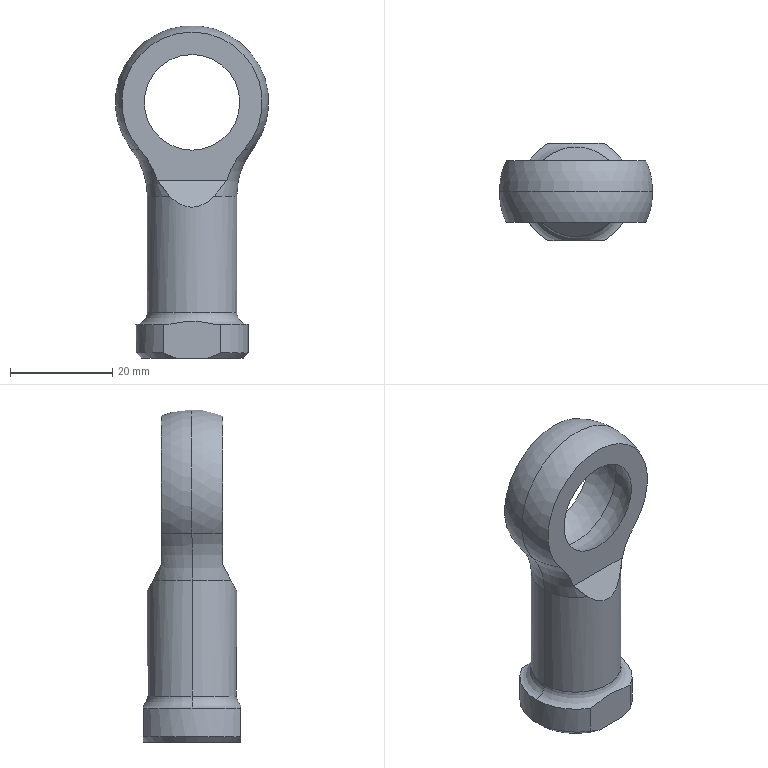Part | NX | 1 solid | 33 faces | box 30 x 19 x 65 mm | volume 11009 mm3 | cylinder 9 | plane 8 | cone 7 | torus 5 | sphere 4 | commonest cylinder face diameters 22 x3 10.096 x2 10.106 x2 17.5 x2